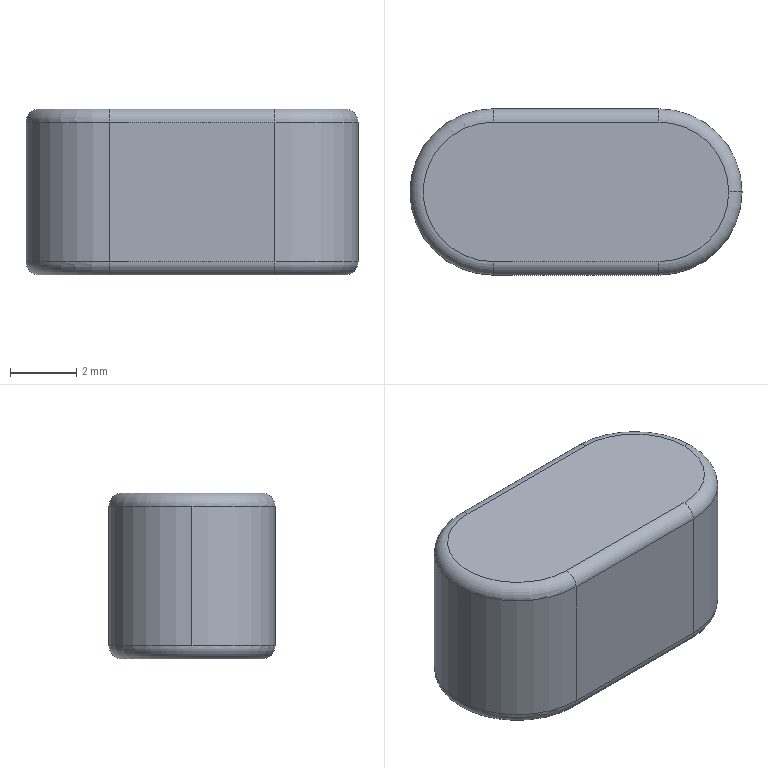Part | SolidWorks | features Extrusion 1, Fillet 1 | 1 solid | 17 faces | box 10 x 5 x 5 mm | volume 221.448 mm3 | cylinder 7 | torus 6 | plane 4 | commonest cylinder face diameters 0.8 x4 5 x3
STEP:
#1=CARTESIAN_POINT('',(4.6,0.,0.));
#2=VERTEX_POINT('',#1);
#3=CARTESIAN_POINT('',(2.5,-2.1,0.));
#4=VERTEX_POINT('',#3);
#5=CARTESIAN_POINT('',(2.5,0.,0.));
#6=DIRECTION('',(0.,0.,-1.));
#7=DIRECTION('',(1.,0.,0.));
#8=AXIS2_PLACEMENT_3D('',#5,#6,#7);
#9=CIRCLE('',#8,2.1);
#10=EDGE_CURVE('',#2,#4,#9,.T.);
#11=ORIENTED_EDGE('',*,*,#10,.F.);
#12=CARTESIAN_POINT('',(5.,0.,0.4));
#13=VERTEX_POINT('',#12);
#14=CARTESIAN_POINT('',(4.6,0.,0.4));
#15=DIRECTION('',(0.,-1.,0.));
#16=DIRECTION('',(0.,0.,-1.));
#17=AXIS2_PLACEMENT_3D('',#14,#15,#16);
#18=CIRCLE('',#17,0.4);
#19=EDGE_CURVE('',#2,#13,#18,.T.);
#20=ORIENTED_EDGE('',*,*,#19,.T.);
#21=CARTESIAN_POINT('',(2.5,-2.5,0.4));
#22=VERTEX_POINT('',#21);
#23=CARTESIAN_POINT('',(2.5,0.,0.4));
#24=DIRECTION('',(0.,0.,1.));
#25=DIRECTION('',(1.,0.,0.));
#26=AXIS2_PLACEMENT_3D('',#23,#24,#25);
#27=CIRCLE('',#26,2.5);
#28=EDGE_CURVE('',#22,#13,#27,.T.);
#29=ORIENTED_EDGE('',*,*,#28,.F.);
#30=CARTESIAN_POINT('',(2.5,-2.1,0.4));
#31=DIRECTION('',(1.,0.,0.));
#32=DIRECTION('',(0.,0.,-1.));
#33=AXIS2_PLACEMENT_3D('',#30,#31,#32);
#34=CIRCLE('',#33,0.4);
#35=EDGE_CURVE('',#22,#4,#34,.T.);
#36=ORIENTED_EDGE('',*,*,#35,.T.);
#37=EDGE_LOOP('',(#11,#20,#29,#36));
#38=FACE_OUTER_BOUND('',#37,.T.);
#39=CARTESIAN_POINT('',(2.5,0.,0.4));
#40=DIRECTION('',(0.,0.,1.));
#41=DIRECTION('',(1.,0.,0.));
#42=AXIS2_PLACEMENT_3D('',#39,#40,#41);
#43=TOROIDAL_SURFACE('',#42,2.1,0.4);
#44=ADVANCED_FACE('',(#38),#43,.T.);
#45=CARTESIAN_POINT('',(5.,0.,4.6));
#46=VERTEX_POINT('',#45);
#47=CARTESIAN_POINT('',(2.5,-2.5,4.6));
#48=VERTEX_POINT('',#47);
#49=CARTESIAN_POINT('',(2.5,0.,4.6));
#50=DIRECTION('',(0.,0.,-1.));
#51=DIRECTION('',(1.,0.,0.));
#52=AXIS2_PLACEMENT_3D('',#49,#50,#51);
#53=CIRCLE('',#52,2.5);
#54=EDGE_CURVE('',#46,#48,#53,.T.);
#55=ORIENTED_EDGE('',*,*,#54,.F.);
#56=CARTESIAN_POINT('',(4.6,0.,5.));
#57=VERTEX_POINT('',#56);
#58=CARTESIAN_POINT('',(4.6,0.,4.6));
#59=DIRECTION('',(0.,-1.,0.));
#60=DIRECTION('',(0.,0.,-1.));
#61=AXIS2_PLACEMENT_3D('',#58,#59,#60);
#62=CIRCLE('',#61,0.4);
#63=EDGE_CURVE('',#46,#57,#62,.T.);
#64=ORIENTED_EDGE('',*,*,#63,.T.);
#65=CARTESIAN_POINT('',(2.5,-2.1,5.));
#66=VERTEX_POINT('',#65);
#67=CARTESIAN_POINT('',(2.5,0.,5.));
#68=DIRECTION('',(0.,0.,1.));
#69=DIRECTION('',(1.,0.,0.));
#70=AXIS2_PLACEMENT_3D('',#67,#68,#69);
#71=CIRCLE('',#70,2.1);
#72=EDGE_CURVE('',#66,#57,#71,.T.);
#73=ORIENTED_EDGE('',*,*,#72,.F.);
#74=CARTESIAN_POINT('',(2.5,-2.1,4.6));
#75=DIRECTION('',(1.,0.,0.));
#76=DIRECTION('',(0.,0.,-1.));
#77=AXIS2_PLACEMENT_3D('',#74,#75,#76);
#78=CIRCLE('',#77,0.4);
#79=EDGE_CURVE('',#66,#48,#78,.T.);
#80=ORIENTED_EDGE('',*,*,#79,.T.);
#81=EDGE_LOOP('',(#55,#64,#73,#80));
#82=FACE_OUTER_BOUND('',#81,.T.);
#83=CARTESIAN_POINT('',(2.5,0.,4.6));
#84=DIRECTION('',(0.,0.,1.));
#85=DIRECTION('',(1.,0.,0.));
#86=AXIS2_PLACEMENT_3D('',#83,#84,#85);
#87=TOROIDAL_SURFACE('',#86,2.1,0.4);
#88=ADVANCED_FACE('',(#82),#87,.T.);
#89=CARTESIAN_POINT('',(-2.5,-2.5,4.6));
#90=VERTEX_POINT('',#89);
#91=CARTESIAN_POINT('',(-5.,0.,4.6));
#92=VERTEX_POINT('',#91);
#93=CARTESIAN_POINT('',(-2.5,0.,4.6));
#94=DIRECTION('',(0.,0.,-1.));
#95=DIRECTION('',(1.,0.,0.));
#96=AXIS2_PLACEMENT_3D('',#93,#94,#95);
#97=CIRCLE('',#96,2.5);
#98=EDGE_CURVE('',#90,#92,#97,.T.);
#99=ORIENTED_EDGE('',*,*,#98,.T.);
#100=CARTESIAN_POINT('',(-5.,0.,0.4));
#101=VERTEX_POINT('',#100);
#102=CARTESIAN_POINT('',(-5.,0.,5.));
#103=DIRECTION('',(0.,0.,-1.));
#104=VECTOR('',#103,1000.);
#105=LINE('',#102,#104);
#106=EDGE_CURVE('',#92,#101,#105,.T.);
#107=ORIENTED_EDGE('',*,*,#106,.T.);
#108=CARTESIAN_POINT('',(-2.5,-2.5,0.4));
#109=VERTEX_POINT('',#108);
#110=CARTESIAN_POINT('',(-2.5,0.,0.4));
#111=DIRECTION('',(0.,0.,1.));
#112=DIRECTION('',(1.,0.,0.));
#113=AXIS2_PLACEMENT_3D('',#110,#111,#112);
#114=CIRCLE('',#113,2.5);
#115=EDGE_CURVE('',#101,#109,#114,.T.);
#116=ORIENTED_EDGE('',*,*,#115,.T.);
#117=CARTESIAN_POINT('',(-2.5,-2.5,5.));
#118=DIRECTION('',(0.,0.,-1.));
#119=VECTOR('',#118,1000.);
#120=LINE('',#117,#119);
#121=EDGE_CURVE('',#90,#109,#120,.T.);
#122=ORIENTED_EDGE('',*,*,#121,.F.);
#123=EDGE_LOOP('',(#99,#107,#116,#122));
#124=FACE_OUTER_BOUND('',#123,.T.);
#125=CARTESIAN_POINT('',(-2.5,0.,5.));
#126=DIRECTION('',(0.,0.,-1.));
#127=DIRECTION('',(-1.,0.,0.));
#128=AXIS2_PLACEMENT_3D('',#125,#126,#127);
#129=CYLINDRICAL_SURFACE('',#128,2.5);
#130=ADVANCED_FACE('',(#124),#129,.T.);
#131=ORIENTED_EDGE('',*,*,#106,.F.);
#132=CARTESIAN_POINT('',(-2.5,2.5,4.6));
#133=VERTEX_POINT('',#132);
#134=CARTESIAN_POINT('',(-2.5,0.,4.6));
#135=DIRECTION('',(0.,0.,-1.));
#136=DIRECTION('',(1.,0.,0.));
#137=AXIS2_PLACEMENT_3D('',#134,#135,#136);
#138=CIRCLE('',#137,2.5);
#139=EDGE_CURVE('',#92,#133,#138,.T.);
#140=ORIENTED_EDGE('',*,*,#139,.T.);
#141=CARTESIAN_POINT('',(-2.5,2.5,0.4));
#142=VERTEX_POINT('',#141);
#143=CARTESIAN_POINT('',(-2.5,2.5,5.));
#144=DIRECTION('',(0.,0.,-1.));
#145=VECTOR('',#144,1000.);
#146=LINE('',#143,#145);
#147=EDGE_CURVE('',#133,#142,#146,.T.);
#148=ORIENTED_EDGE('',*,*,#147,.T.);
#149=CARTESIAN_POINT('',(-2.5,0.,0.4));
#150=DIRECTION('',(0.,0.,1.));
#151=DIRECTION('',(1.,0.,0.));
#152=AXIS2_PLACEMENT_3D('',#149,#150,#151);
#153=CIRCLE('',#152,2.5);
#154=EDGE_CURVE('',#142,#101,#153,.T.);
#155=ORIENTED_EDGE('',*,*,#154,.T.);
#156=EDGE_LOOP('',(#131,#140,#148,#155));
#157=FACE_OUTER_BOUND('',#156,.T.);
#158=CARTESIAN_POINT('',(-2.5,0.,5.));
#159=DIRECTION('',(0.,0.,-1.));
#160=DIRECTION('',(-1.,0.,0.));
#161=AXIS2_PLACEMENT_3D('',#158,#159,#160);
#162=CYLINDRICAL_SURFACE('',#161,2.5);
#163=ADVANCED_FACE('',(#157),#162,.T.);
#164=CARTESIAN_POINT('',(2.5,-2.5,5.));
#165=DIRECTION('',(0.,0.,-1.));
#166=VECTOR('',#165,1000.);
#167=LINE('',#164,#166);
#168=EDGE_CURVE('',#48,#22,#167,.T.);
#169=ORIENTED_EDGE('',*,*,#168,.F.);
#170=CARTESIAN_POINT('',(-2.5,-2.5,4.6));
#171=DIRECTION('',(-1.,0.,0.));
#172=VECTOR('',#171,1000.);
#173=LINE('',#170,#172);
#174=EDGE_CURVE('',#48,#90,#173,.T.);
#175=ORIENTED_EDGE('',*,*,#174,.T.);
#176=ORIENTED_EDGE('',*,*,#121,.T.);
#177=CARTESIAN_POINT('',(-2.5,-2.5,0.4));
#178=DIRECTION('',(1.,0.,0.));
#179=VECTOR('',#178,1000.);
#180=LINE('',#177,#179);
#181=EDGE_CURVE('',#109,#22,#180,.T.);
#182=ORIENTED_EDGE('',*,*,#181,.T.);
#183=EDGE_LOOP('',(#169,#175,#176,#182));
#184=FACE_OUTER_BOUND('',#183,.T.);
#185=CARTESIAN_POINT('',(-2.5,-2.5,5.));
#186=DIRECTION('',(0.,1.,0.));
#187=DIRECTION('',(-1.,0.,0.));
#188=AXIS2_PLACEMENT_3D('',#185,#186,#187);
#189=PLANE('',#188);
#190=ADVANCED_FACE('',(#184),#189,.F.);
#191=CARTESIAN_POINT('',(2.5,2.5,4.6));
#192=VERTEX_POINT('',#191);
#193=CARTESIAN_POINT('',(2.5,2.5,0.4));
#194=VERTEX_POINT('',#193);
#195=CARTESIAN_POINT('',(2.5,2.5,5.));
#196=DIRECTION('',(0.,0.,-1.));
#197=VECTOR('',#196,1000.);
#198=LINE('',#195,#197);
#199=EDGE_CURVE('',#192,#194,#198,.T.);
#200=ORIENTED_EDGE('',*,*,#199,.F.);
#201=CARTESIAN_POINT('',(2.5,0.,4.6));
#202=DIRECTION('',(0.,0.,-1.));
#203=DIRECTION('',(1.,0.,0.));
#204=AXIS2_PLACEMENT_3D('',#201,#202,#203);
#205=CIRCLE('',#204,2.5);
#206=EDGE_CURVE('',#192,#46,#205,.T.);
#207=ORIENTED_EDGE('',*,*,#206,.T.);
#208=ORIENTED_EDGE('',*,*,#54,.T.);
#209=ORIENTED_EDGE('',*,*,#168,.T.);
#210=ORIENTED_EDGE('',*,*,#28,.T.);
#211=CARTESIAN_POINT('',(2.5,0.,0.4));
#212=DIRECTION('',(0.,0.,1.));
#213=DIRECTION('',(1.,0.,0.));
#214=AXIS2_PLACEMENT_3D('',#211,#212,#213);
#215=CIRCLE('',#214,2.5);
#216=EDGE_CURVE('',#13,#194,#215,.T.);
#217=ORIENTED_EDGE('',*,*,#216,.T.);
#218=EDGE_LOOP('',(#200,#207,#208,#209,#210,#217));
#219=FACE_OUTER_BOUND('',#218,.T.);
#220=CARTESIAN_POINT('',(2.5,0.,5.));
#221=DIRECTION('',(0.,0.,-1.));
#222=DIRECTION('',(-1.,0.,0.));
#223=AXIS2_PLACEMENT_3D('',#220,#221,#222);
#224=CYLINDRICAL_SURFACE('',#223,2.5);
#225=ADVANCED_FACE('',(#219),#224,.T.);
#226=ORIENTED_EDGE('',*,*,#147,.F.);
#227=CARTESIAN_POINT('',(2.5,2.5,4.6));
#228=DIRECTION('',(1.,0.,0.));
#229=VECTOR('',#228,1000.);
#230=LINE('',#227,#229);
#231=EDGE_CURVE('',#133,#192,#230,.T.);
#232=ORIENTED_EDGE('',*,*,#231,.T.);
#233=ORIENTED_EDGE('',*,*,#199,.T.);
#234=CARTESIAN_POINT('',(-2.5,2.5,0.4));
#235=DIRECTION('',(-1.,0.,0.));
#236=VECTOR('',#235,1000.);
#237=LINE('',#234,#236);
#238=EDGE_CURVE('',#194,#142,#237,.T.);
#239=ORIENTED_EDGE('',*,*,#238,.T.);
#240=EDGE_LOOP('',(#226,#232,#233,#239));
#241=FACE_OUTER_BOUND('',#240,.T.);
#242=CARTESIAN_POINT('',(-2.5,2.5,5.));
#243=DIRECTION('',(0.,-1.,0.));
#244=DIRECTION('',(1.,0.,0.));
#245=AXIS2_PLACEMENT_3D('',#242,#243,#244);
#246=PLANE('',#245);
#247=ADVANCED_FACE('',(#241),#246,.F.);
#248=CARTESIAN_POINT('',(-2.5,-2.1,5.));
#249=VERTEX_POINT('',#248);
#250=CARTESIAN_POINT('',(2.5,-2.1,5.));
#251=DIRECTION('',(1.,0.,0.));
#252=VECTOR('',#251,1000.);
#253=LINE('',#250,#252);
#254=EDGE_CURVE('',#249,#66,#253,.T.);
#255=ORIENTED_EDGE('',*,*,#254,.T.);
#256=ORIENTED_EDGE('',*,*,#72,.T.);
#257=CARTESIAN_POINT('',(2.5,2.1,5.));
#258=VERTEX_POINT('',#257);
#259=CARTESIAN_POINT('',(2.5,0.,5.));
#260=DIRECTION('',(0.,0.,1.));
#261=DIRECTION('',(1.,0.,0.));
#262=AXIS2_PLACEMENT_3D('',#259,#260,#261);
#263=CIRCLE('',#262,2.1);
#264=EDGE_CURVE('',#57,#258,#263,.T.);
#265=ORIENTED_EDGE('',*,*,#264,.T.);
#266=CARTESIAN_POINT('',(-2.5,2.1,5.));
#267=VERTEX_POINT('',#266);
#268=CARTESIAN_POINT('',(-2.5,2.1,5.));
#269=DIRECTION('',(-1.,0.,0.));
#270=VECTOR('',#269,1000.);
#271=LINE('',#268,#270);
#272=EDGE_CURVE('',#258,#267,#271,.T.);
#273=ORIENTED_EDGE('',*,*,#272,.T.);
#274=CARTESIAN_POINT('',(-2.5,0.,5.));
#275=DIRECTION('',(0.,0.,1.));
#276=DIRECTION('',(1.,0.,0.));
#277=AXIS2_PLACEMENT_3D('',#274,#275,#276);
#278=CIRCLE('',#277,2.1);
#279=EDGE_CURVE('',#267,#249,#278,.T.);
#280=ORIENTED_EDGE('',*,*,#279,.T.);
#281=EDGE_LOOP('',(#255,#256,#265,#273,#280));
#282=FACE_OUTER_BOUND('',#281,.T.);
#283=CARTESIAN_POINT('',(-2.5,0.,5.));
#284=DIRECTION('',(0.,0.,1.));
#285=DIRECTION('',(1.,0.,0.));
#286=AXIS2_PLACEMENT_3D('',#283,#284,#285);
#287=PLANE('',#286);
#288=ADVANCED_FACE('',(#282),#287,.T.);
#289=CARTESIAN_POINT('',(-2.5,2.1,0.));
#290=VERTEX_POINT('',#289);
#291=CARTESIAN_POINT('',(2.5,2.1,0.));
#292=VERTEX_POINT('',#291);
#293=CARTESIAN_POINT('',(-2.5,2.1,0.));
#294=DIRECTION('',(1.,0.,0.));
#295=VECTOR('',#294,1000.);
#296=LINE('',#293,#295);
#297=EDGE_CURVE('',#290,#292,#296,.T.);
#298=ORIENTED_EDGE('',*,*,#297,.T.);
#299=CARTESIAN_POINT('',(2.5,0.,0.));
#300=DIRECTION('',(0.,0.,-1.));
#301=DIRECTION('',(1.,0.,0.));
#302=AXIS2_PLACEMENT_3D('',#299,#300,#301);
#303=CIRCLE('',#302,2.1);
#304=EDGE_CURVE('',#292,#2,#303,.T.);
#305=ORIENTED_EDGE('',*,*,#304,.T.);
#306=ORIENTED_EDGE('',*,*,#10,.T.);
#307=CARTESIAN_POINT('',(-2.5,-2.1,0.));
#308=VERTEX_POINT('',#307);
#309=CARTESIAN_POINT('',(-2.5,-2.1,0.));
#310=DIRECTION('',(-1.,0.,0.));
#311=VECTOR('',#310,1000.);
#312=LINE('',#309,#311);
#313=EDGE_CURVE('',#4,#308,#312,.T.);
#314=ORIENTED_EDGE('',*,*,#313,.T.);
#315=CARTESIAN_POINT('',(-2.5,0.,0.));
#316=DIRECTION('',(0.,0.,-1.));
#317=DIRECTION('',(1.,0.,0.));
#318=AXIS2_PLACEMENT_3D('',#315,#316,#317);
#319=CIRCLE('',#318,2.1);
#320=EDGE_CURVE('',#308,#290,#319,.T.);
#321=ORIENTED_EDGE('',*,*,#320,.T.);
#322=EDGE_LOOP('',(#298,#305,#306,#314,#321));
#323=FACE_OUTER_BOUND('',#322,.T.);
#324=CARTESIAN_POINT('',(-2.5,0.,0.));
#325=DIRECTION('',(0.,0.,1.));
#326=DIRECTION('',(1.,0.,0.));
#327=AXIS2_PLACEMENT_3D('',#324,#325,#326);
#328=PLANE('',#327);
#329=ADVANCED_FACE('',(#323),#328,.F.);
#330=CARTESIAN_POINT('',(-2.5,2.1,4.6));
#331=DIRECTION('',(1.,0.,0.));
#332=DIRECTION('',(0.,0.,-1.));
#333=AXIS2_PLACEMENT_3D('',#330,#331,#332);
#334=CIRCLE('',#333,0.4);
#335=EDGE_CURVE('',#133,#267,#334,.T.);
#336=ORIENTED_EDGE('',*,*,#335,.F.);
#337=ORIENTED_EDGE('',*,*,#139,.F.);
#338=ORIENTED_EDGE('',*,*,#98,.F.);
#339=CARTESIAN_POINT('',(-2.5,-2.1,4.6));
#340=DIRECTION('',(1.,0.,0.));
#341=DIRECTION('',(0.,0.,-1.));
#342=AXIS2_PLACEMENT_3D('',#339,#340,#341);
#343=CIRCLE('',#342,0.4);
#344=EDGE_CURVE('',#249,#90,#343,.T.);
#345=ORIENTED_EDGE('',*,*,#344,.F.);
#346=ORIENTED_EDGE('',*,*,#279,.F.);
#347=EDGE_LOOP('',(#336,#337,#338,#345,#346));
#348=FACE_OUTER_BOUND('',#347,.T.);
#349=CARTESIAN_POINT('',(-2.5,0.,4.6));
#350=DIRECTION('',(0.,0.,1.));
#351=DIRECTION('',(1.,0.,0.));
#352=AXIS2_PLACEMENT_3D('',#349,#350,#351);
#353=TOROIDAL_SURFACE('',#352,2.1,0.4);
#354=ADVANCED_FACE('',(#348),#353,.T.);
#355=ORIENTED_EDGE('',*,*,#344,.T.);
#356=ORIENTED_EDGE('',*,*,#174,.F.);
#357=ORIENTED_EDGE('',*,*,#79,.F.);
#358=ORIENTED_EDGE('',*,*,#254,.F.);
#359=EDGE_LOOP('',(#355,#356,#357,#358));
#360=FACE_OUTER_BOUND('',#359,.T.);
#361=CARTESIAN_POINT('',(-2.5,-2.1,4.6));
#362=DIRECTION('',(-1.,0.,0.));
#363=DIRECTION('',(0.,-1.,0.));
#364=AXIS2_PLACEMENT_3D('',#361,#362,#363);
#365=CYLINDRICAL_SURFACE('',#364,0.4);
#366=ADVANCED_FACE('',(#360),#365,.T.);
#367=ORIENTED_EDGE('',*,*,#335,.T.);
#368=ORIENTED_EDGE('',*,*,#272,.F.);
#369=CARTESIAN_POINT('',(2.5,2.1,4.6));
#370=DIRECTION('',(1.,0.,0.));
#371=DIRECTION('',(0.,0.,-1.));
#372=AXIS2_PLACEMENT_3D('',#369,#370,#371);
#373=CIRCLE('',#372,0.4);
#374=EDGE_CURVE('',#192,#258,#373,.T.);
#375=ORIENTED_EDGE('',*,*,#374,.F.);
#376=ORIENTED_EDGE('',*,*,#231,.F.);
#377=EDGE_LOOP('',(#367,#368,#375,#376));
#378=FACE_OUTER_BOUND('',#377,.T.);
#379=CARTESIAN_POINT('',(-2.5,2.1,4.6));
#380=DIRECTION('',(1.,0.,0.));
#381=DIRECTION('',(0.,1.,0.));
#382=AXIS2_PLACEMENT_3D('',#379,#380,#381);
#383=CYLINDRICAL_SURFACE('',#382,0.4);
#384=ADVANCED_FACE('',(#378),#383,.T.);
#385=ORIENTED_EDGE('',*,*,#63,.F.);
#386=ORIENTED_EDGE('',*,*,#206,.F.);
#387=ORIENTED_EDGE('',*,*,#374,.T.);
#388=ORIENTED_EDGE('',*,*,#264,.F.);
#389=EDGE_LOOP('',(#385,#386,#387,#388));
#390=FACE_OUTER_BOUND('',#389,.T.);
#391=CARTESIAN_POINT('',(2.5,0.,4.6));
#392=DIRECTION('',(0.,0.,1.));
#393=DIRECTION('',(1.,0.,0.));
#394=AXIS2_PLACEMENT_3D('',#391,#392,#393);
#395=TOROIDAL_SURFACE('',#394,2.1,0.4);
#396=ADVANCED_FACE('',(#390),#395,.T.);
#397=CARTESIAN_POINT('',(-2.5,2.1,0.4));
#398=DIRECTION('',(1.,0.,0.));
#399=DIRECTION('',(0.,0.,-1.));
#400=AXIS2_PLACEMENT_3D('',#397,#398,#399);
#401=CIRCLE('',#400,0.4);
#402=EDGE_CURVE('',#290,#142,#401,.T.);
#403=ORIENTED_EDGE('',*,*,#402,.F.);
#404=ORIENTED_EDGE('',*,*,#320,.F.);
#405=CARTESIAN_POINT('',(-2.5,-2.1,0.4));
#406=DIRECTION('',(1.,0.,0.));
#407=DIRECTION('',(0.,0.,-1.));
#408=AXIS2_PLACEMENT_3D('',#405,#406,#407);
#409=CIRCLE('',#408,0.4);
#410=EDGE_CURVE('',#109,#308,#409,.T.);
#411=ORIENTED_EDGE('',*,*,#410,.F.);
#412=ORIENTED_EDGE('',*,*,#115,.F.);
#413=ORIENTED_EDGE('',*,*,#154,.F.);
#414=EDGE_LOOP('',(#403,#404,#411,#412,#413));
#415=FACE_OUTER_BOUND('',#414,.T.);
#416=CARTESIAN_POINT('',(-2.5,0.,0.4));
#417=DIRECTION('',(0.,0.,1.));
#418=DIRECTION('',(1.,0.,0.));
#419=AXIS2_PLACEMENT_3D('',#416,#417,#418);
#420=TOROIDAL_SURFACE('',#419,2.1,0.4);
#421=ADVANCED_FACE('',(#415),#420,.T.);
#422=ORIENTED_EDGE('',*,*,#410,.T.);
#423=ORIENTED_EDGE('',*,*,#313,.F.);
#424=ORIENTED_EDGE('',*,*,#35,.F.);
#425=ORIENTED_EDGE('',*,*,#181,.F.);
#426=EDGE_LOOP('',(#422,#423,#424,#425));
#427=FACE_OUTER_BOUND('',#426,.T.);
#428=CARTESIAN_POINT('',(-2.5,-2.1,0.4));
#429=DIRECTION('',(1.,0.,0.));
#430=DIRECTION('',(0.,1.,0.));
#431=AXIS2_PLACEMENT_3D('',#428,#429,#430);
#432=CYLINDRICAL_SURFACE('',#431,0.4);
#433=ADVANCED_FACE('',(#427),#432,.T.);
#434=ORIENTED_EDGE('',*,*,#402,.T.);
#435=ORIENTED_EDGE('',*,*,#238,.F.);
#436=CARTESIAN_POINT('',(2.5,2.1,0.4));
#437=DIRECTION('',(1.,0.,0.));
#438=DIRECTION('',(0.,0.,-1.));
#439=AXIS2_PLACEMENT_3D('',#436,#437,#438);
#440=CIRCLE('',#439,0.4);
#441=EDGE_CURVE('',#292,#194,#440,.T.);
#442=ORIENTED_EDGE('',*,*,#441,.F.);
#443=ORIENTED_EDGE('',*,*,#297,.F.);
#444=EDGE_LOOP('',(#434,#435,#442,#443));
#445=FACE_OUTER_BOUND('',#444,.T.);
#446=CARTESIAN_POINT('',(-2.5,2.1,0.4));
#447=DIRECTION('',(-1.,0.,0.));
#448=DIRECTION('',(0.,-1.,0.));
#449=AXIS2_PLACEMENT_3D('',#446,#447,#448);
#450=CYLINDRICAL_SURFACE('',#449,0.4);
#451=ADVANCED_FACE('',(#445),#450,.T.);
#452=ORIENTED_EDGE('',*,*,#19,.F.);
#453=ORIENTED_EDGE('',*,*,#304,.F.);
#454=ORIENTED_EDGE('',*,*,#441,.T.);
#455=ORIENTED_EDGE('',*,*,#216,.F.);
#456=EDGE_LOOP('',(#452,#453,#454,#455));
#457=FACE_OUTER_BOUND('',#456,.T.);
#458=CARTESIAN_POINT('',(2.5,0.,0.4));
#459=DIRECTION('',(0.,0.,1.));
#460=DIRECTION('',(1.,0.,0.));
#461=AXIS2_PLACEMENT_3D('',#458,#459,#460);
#462=TOROIDAL_SURFACE('',#461,2.1,0.4);
#463=ADVANCED_FACE('',(#457),#462,.T.);
#464=CLOSED_SHELL('',(#44,#88,#130,#163,#190,#225,#247,#288,#329,#354,#366,#384,#396,#421,#433,#451,#463));
#465=MANIFOLD_SOLID_BREP('',#464);
#466=CARTESIAN_POINT('',(0.,0.,0.));
#467=DIRECTION('',(0.,0.,1.));
#468=DIRECTION('',(1.,0.,0.));
#469=AXIS2_PLACEMENT_3D('',#466,#467,#468);
#470=(LENGTH_UNIT()NAMED_UNIT(*)SI_UNIT(.MILLI.,.METRE.));
#471=UNCERTAINTY_MEASURE_WITH_UNIT(LENGTH_MEASURE(0.00001),#470,'','');
#472=(NAMED_UNIT(*)PLANE_ANGLE_UNIT()SI_UNIT($,.RADIAN.));
#473=(NAMED_UNIT(*)SI_UNIT($,.STERADIAN.)SOLID_ANGLE_UNIT());
#474=(GEOMETRIC_REPRESENTATION_CONTEXT(3)GLOBAL_UNCERTAINTY_ASSIGNED_CONTEXT((#471))GLOBAL_UNIT_ASSIGNED_CONTEXT((#470,#472,#473))REPRESENTATION_CONTEXT('',''));
#475=ADVANCED_BREP_SHAPE_REPRESENTATION('',(#465,#469),#474);